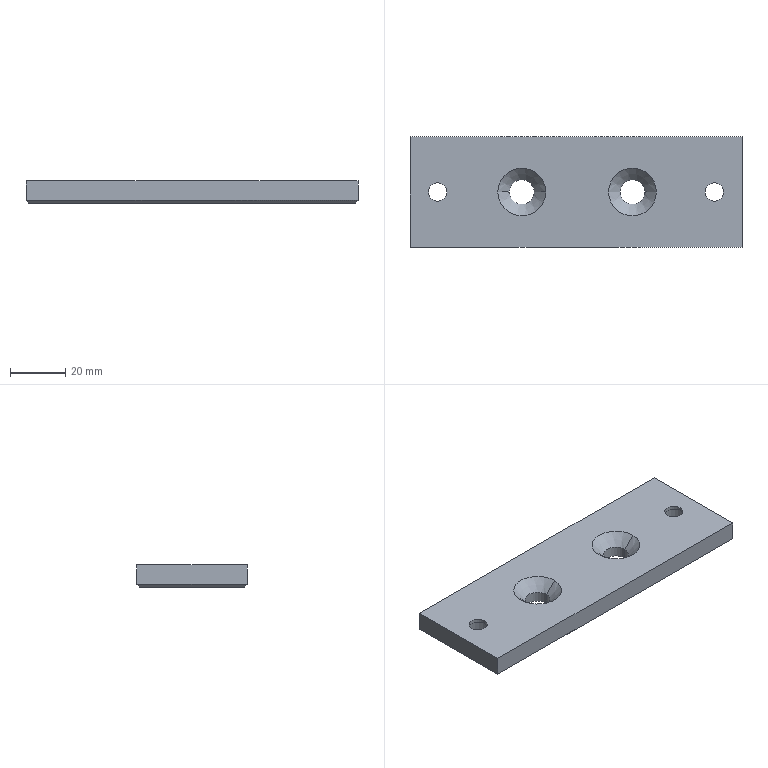Part | SolidWorks | features 3DProfileFeature 2, HoleWzd 2, Chamfer 1, Extrusion 1 | 1 solid | 28 faces | box 120 x 40 x 8 mm | volume 35212 mm3 | cylinder 12 | plane 12 | cone 4 | commonest cylinder face diameters 6.6 x4 9 x4 11 x4
STEP:
#1=CARTESIAN_POINT('',(55.5,0.,2.8));
#2=VERTEX_POINT('',#1);
#3=CARTESIAN_POINT('',(44.5,0.,2.8));
#4=VERTEX_POINT('',#3);
#5=CARTESIAN_POINT('',(50.,0.,2.8));
#6=DIRECTION('',(0.,0.,-1.));
#7=DIRECTION('',(-1.,0.,0.));
#8=AXIS2_PLACEMENT_3D('',#5,#6,#7);
#9=CIRCLE('',#8,5.5);
#10=EDGE_CURVE('',#2,#4,#9,.T.);
#11=ORIENTED_EDGE('',*,*,#10,.F.);
#12=CARTESIAN_POINT('',(55.5,0.,-4.));
#13=VERTEX_POINT('',#12);
#14=CARTESIAN_POINT('',(55.5,0.,-4.));
#15=DIRECTION('',(0.,0.,-1.));
#16=VECTOR('',#15,1000.);
#17=LINE('',#14,#16);
#18=EDGE_CURVE('',#2,#13,#17,.T.);
#19=ORIENTED_EDGE('',*,*,#18,.T.);
#20=CARTESIAN_POINT('',(44.5,0.,-4.));
#21=VERTEX_POINT('',#20);
#22=CARTESIAN_POINT('',(50.,0.,-4.));
#23=DIRECTION('',(0.,0.,-1.));
#24=DIRECTION('',(-1.,0.,0.));
#25=AXIS2_PLACEMENT_3D('',#22,#23,#24);
#26=CIRCLE('',#25,5.5);
#27=EDGE_CURVE('',#13,#21,#26,.T.);
#28=ORIENTED_EDGE('',*,*,#27,.T.);
#29=CARTESIAN_POINT('',(44.5,0.,-4.));
#30=DIRECTION('',(0.,0.,-1.));
#31=VECTOR('',#30,1000.);
#32=LINE('',#29,#31);
#33=EDGE_CURVE('',#4,#21,#32,.T.);
#34=ORIENTED_EDGE('',*,*,#33,.F.);
#35=EDGE_LOOP('',(#11,#19,#28,#34));
#36=FACE_OUTER_BOUND('',#35,.T.);
#37=CARTESIAN_POINT('',(50.,0.,-4.));
#38=DIRECTION('',(0.,0.,-1.));
#39=DIRECTION('',(-1.,0.,0.));
#40=AXIS2_PLACEMENT_3D('',#37,#38,#39);
#41=CYLINDRICAL_SURFACE('',#40,5.5);
#42=ADVANCED_FACE('',(#36),#41,.F.);
#43=CARTESIAN_POINT('',(46.7,0.,4.));
#44=VERTEX_POINT('',#43);
#45=CARTESIAN_POINT('',(53.3,0.,4.));
#46=VERTEX_POINT('',#45);
#47=CARTESIAN_POINT('',(50.,0.,4.));
#48=DIRECTION('',(0.,0.,1.));
#49=DIRECTION('',(1.,0.,0.));
#50=AXIS2_PLACEMENT_3D('',#47,#48,#49);
#51=CIRCLE('',#50,3.3);
#52=EDGE_CURVE('',#44,#46,#51,.T.);
#53=ORIENTED_EDGE('',*,*,#52,.T.);
#54=CARTESIAN_POINT('',(53.3,0.,2.8));
#55=VERTEX_POINT('',#54);
#56=CARTESIAN_POINT('',(53.3,0.,-4.));
#57=DIRECTION('',(0.,0.,-1.));
#58=VECTOR('',#57,1000.);
#59=LINE('',#56,#58);
#60=EDGE_CURVE('',#46,#55,#59,.T.);
#61=ORIENTED_EDGE('',*,*,#60,.T.);
#62=CARTESIAN_POINT('',(46.7,0.,2.8));
#63=VERTEX_POINT('',#62);
#64=CARTESIAN_POINT('',(50.,0.,2.8));
#65=DIRECTION('',(0.,0.,-1.));
#66=DIRECTION('',(-1.,0.,0.));
#67=AXIS2_PLACEMENT_3D('',#64,#65,#66);
#68=CIRCLE('',#67,3.3);
#69=EDGE_CURVE('',#55,#63,#68,.T.);
#70=ORIENTED_EDGE('',*,*,#69,.T.);
#71=CARTESIAN_POINT('',(46.7,0.,-4.));
#72=DIRECTION('',(0.,0.,-1.));
#73=VECTOR('',#72,1000.);
#74=LINE('',#71,#73);
#75=EDGE_CURVE('',#44,#63,#74,.T.);
#76=ORIENTED_EDGE('',*,*,#75,.F.);
#77=EDGE_LOOP('',(#53,#61,#70,#76));
#78=FACE_OUTER_BOUND('',#77,.T.);
#79=CARTESIAN_POINT('',(50.,0.,-4.));
#80=DIRECTION('',(0.,0.,-1.));
#81=DIRECTION('',(-1.,0.,0.));
#82=AXIS2_PLACEMENT_3D('',#79,#80,#81);
#83=CYLINDRICAL_SURFACE('',#82,3.3);
#84=ADVANCED_FACE('',(#78),#83,.F.);
#85=CARTESIAN_POINT('',(-44.5,0.,2.8));
#86=VERTEX_POINT('',#85);
#87=CARTESIAN_POINT('',(-55.5,0.,2.8));
#88=VERTEX_POINT('',#87);
#89=CARTESIAN_POINT('',(-50.,0.,2.8));
#90=DIRECTION('',(0.,0.,-1.));
#91=DIRECTION('',(-1.,0.,0.));
#92=AXIS2_PLACEMENT_3D('',#89,#90,#91);
#93=CIRCLE('',#92,5.5);
#94=EDGE_CURVE('',#86,#88,#93,.T.);
#95=ORIENTED_EDGE('',*,*,#94,.F.);
#96=CARTESIAN_POINT('',(-44.5,0.,-4.));
#97=VERTEX_POINT('',#96);
#98=CARTESIAN_POINT('',(-44.5,0.,-4.));
#99=DIRECTION('',(0.,0.,-1.));
#100=VECTOR('',#99,1000.);
#101=LINE('',#98,#100);
#102=EDGE_CURVE('',#86,#97,#101,.T.);
#103=ORIENTED_EDGE('',*,*,#102,.T.);
#104=CARTESIAN_POINT('',(-55.5,0.,-4.));
#105=VERTEX_POINT('',#104);
#106=CARTESIAN_POINT('',(-50.,0.,-4.));
#107=DIRECTION('',(0.,0.,-1.));
#108=DIRECTION('',(-1.,0.,0.));
#109=AXIS2_PLACEMENT_3D('',#106,#107,#108);
#110=CIRCLE('',#109,5.5);
#111=EDGE_CURVE('',#97,#105,#110,.T.);
#112=ORIENTED_EDGE('',*,*,#111,.T.);
#113=CARTESIAN_POINT('',(-55.5,0.,-4.));
#114=DIRECTION('',(0.,0.,-1.));
#115=VECTOR('',#114,1000.);
#116=LINE('',#113,#115);
#117=EDGE_CURVE('',#88,#105,#116,.T.);
#118=ORIENTED_EDGE('',*,*,#117,.F.);
#119=EDGE_LOOP('',(#95,#103,#112,#118));
#120=FACE_OUTER_BOUND('',#119,.T.);
#121=CARTESIAN_POINT('',(-50.,0.,-4.));
#122=DIRECTION('',(0.,0.,-1.));
#123=DIRECTION('',(-1.,0.,0.));
#124=AXIS2_PLACEMENT_3D('',#121,#122,#123);
#125=CYLINDRICAL_SURFACE('',#124,5.5);
#126=ADVANCED_FACE('',(#120),#125,.F.);
#127=CARTESIAN_POINT('',(-53.3,0.,4.));
#128=VERTEX_POINT('',#127);
#129=CARTESIAN_POINT('',(-46.7,0.,4.));
#130=VERTEX_POINT('',#129);
#131=CARTESIAN_POINT('',(-50.,0.,4.));
#132=DIRECTION('',(0.,0.,1.));
#133=DIRECTION('',(1.,0.,0.));
#134=AXIS2_PLACEMENT_3D('',#131,#132,#133);
#135=CIRCLE('',#134,3.3);
#136=EDGE_CURVE('',#128,#130,#135,.T.);
#137=ORIENTED_EDGE('',*,*,#136,.T.);
#138=CARTESIAN_POINT('',(-46.7,0.,2.8));
#139=VERTEX_POINT('',#138);
#140=CARTESIAN_POINT('',(-46.7,0.,-4.));
#141=DIRECTION('',(0.,0.,-1.));
#142=VECTOR('',#141,1000.);
#143=LINE('',#140,#142);
#144=EDGE_CURVE('',#130,#139,#143,.T.);
#145=ORIENTED_EDGE('',*,*,#144,.T.);
#146=CARTESIAN_POINT('',(-53.3,0.,2.8));
#147=VERTEX_POINT('',#146);
#148=CARTESIAN_POINT('',(-50.,0.,2.8));
#149=DIRECTION('',(0.,0.,-1.));
#150=DIRECTION('',(-1.,0.,0.));
#151=AXIS2_PLACEMENT_3D('',#148,#149,#150);
#152=CIRCLE('',#151,3.3);
#153=EDGE_CURVE('',#139,#147,#152,.T.);
#154=ORIENTED_EDGE('',*,*,#153,.T.);
#155=CARTESIAN_POINT('',(-53.3,0.,-4.));
#156=DIRECTION('',(0.,0.,-1.));
#157=VECTOR('',#156,1000.);
#158=LINE('',#155,#157);
#159=EDGE_CURVE('',#128,#147,#158,.T.);
#160=ORIENTED_EDGE('',*,*,#159,.F.);
#161=EDGE_LOOP('',(#137,#145,#154,#160));
#162=FACE_OUTER_BOUND('',#161,.T.);
#163=CARTESIAN_POINT('',(-50.,0.,-4.));
#164=DIRECTION('',(0.,0.,-1.));
#165=DIRECTION('',(-1.,0.,0.));
#166=AXIS2_PLACEMENT_3D('',#163,#164,#165);
#167=CYLINDRICAL_SURFACE('',#166,3.3);
#168=ADVANCED_FACE('',(#162),#167,.F.);
#169=CARTESIAN_POINT('',(-24.096,0.,-0.15));
#170=VERTEX_POINT('',#169);
#171=CARTESIAN_POINT('',(-15.096,0.,-0.15));
#172=VERTEX_POINT('',#171);
#173=CARTESIAN_POINT('',(-19.596,0.,-0.15));
#174=DIRECTION('',(0.,0.,1.));
#175=DIRECTION('',(1.,0.,0.));
#176=AXIS2_PLACEMENT_3D('',#173,#174,#175);
#177=CIRCLE('',#176,4.5);
#178=EDGE_CURVE('',#170,#172,#177,.T.);
#179=ORIENTED_EDGE('',*,*,#178,.F.);
#180=CARTESIAN_POINT('',(-28.246,0.,4.));
#181=VERTEX_POINT('',#180);
#182=CARTESIAN_POINT('',(-28.246,0.,4.));
#183=DIRECTION('',(-0.7071,0.,0.7071));
#184=VECTOR('',#183,1000.);
#185=LINE('',#182,#184);
#186=EDGE_CURVE('',#170,#181,#185,.T.);
#187=ORIENTED_EDGE('',*,*,#186,.T.);
#188=CARTESIAN_POINT('',(-10.946,0.,4.));
#189=VERTEX_POINT('',#188);
#190=CARTESIAN_POINT('',(-19.596,0.,4.));
#191=DIRECTION('',(0.,0.,1.));
#192=DIRECTION('',(1.,0.,0.));
#193=AXIS2_PLACEMENT_3D('',#190,#191,#192);
#194=CIRCLE('',#193,8.65);
#195=EDGE_CURVE('',#181,#189,#194,.T.);
#196=ORIENTED_EDGE('',*,*,#195,.T.);
#197=CARTESIAN_POINT('',(-10.946,0.,4.));
#198=DIRECTION('',(0.7071,0.,0.7071));
#199=VECTOR('',#198,1000.);
#200=LINE('',#197,#199);
#201=EDGE_CURVE('',#172,#189,#200,.T.);
#202=ORIENTED_EDGE('',*,*,#201,.F.);
#203=EDGE_LOOP('',(#179,#187,#196,#202));
#204=FACE_OUTER_BOUND('',#203,.T.);
#205=CARTESIAN_POINT('',(-19.596,0.,4.));
#206=DIRECTION('',(0.,0.,1.));
#207=DIRECTION('',(1.,0.,0.));
#208=AXIS2_PLACEMENT_3D('',#205,#206,#207);
#209=CONICAL_SURFACE('',#208,8.65,0.7854);
#210=ADVANCED_FACE('',(#204),#209,.F.);
#211=CARTESIAN_POINT('',(-24.096,0.,-4.));
#212=VERTEX_POINT('',#211);
#213=CARTESIAN_POINT('',(-15.096,0.,-4.));
#214=VERTEX_POINT('',#213);
#215=CARTESIAN_POINT('',(-19.596,0.,-4.));
#216=DIRECTION('',(0.,0.,1.));
#217=DIRECTION('',(1.,0.,0.));
#218=AXIS2_PLACEMENT_3D('',#215,#216,#217);
#219=CIRCLE('',#218,4.5);
#220=EDGE_CURVE('',#212,#214,#219,.T.);
#221=ORIENTED_EDGE('',*,*,#220,.F.);
#222=CARTESIAN_POINT('',(-24.096,0.,4.));
#223=DIRECTION('',(0.,0.,1.));
#224=VECTOR('',#223,1000.);
#225=LINE('',#222,#224);
#226=EDGE_CURVE('',#212,#170,#225,.T.);
#227=ORIENTED_EDGE('',*,*,#226,.T.);
#228=ORIENTED_EDGE('',*,*,#178,.T.);
#229=CARTESIAN_POINT('',(-15.096,0.,4.));
#230=DIRECTION('',(0.,0.,1.));
#231=VECTOR('',#230,1000.);
#232=LINE('',#229,#231);
#233=EDGE_CURVE('',#214,#172,#232,.T.);
#234=ORIENTED_EDGE('',*,*,#233,.F.);
#235=EDGE_LOOP('',(#221,#227,#228,#234));
#236=FACE_OUTER_BOUND('',#235,.T.);
#237=CARTESIAN_POINT('',(-19.596,0.,4.));
#238=DIRECTION('',(0.,0.,1.));
#239=DIRECTION('',(1.,0.,0.));
#240=AXIS2_PLACEMENT_3D('',#237,#238,#239);
#241=CYLINDRICAL_SURFACE('',#240,4.5);
#242=ADVANCED_FACE('',(#236),#241,.F.);
#243=CARTESIAN_POINT('',(15.904,0.,-0.15));
#244=VERTEX_POINT('',#243);
#245=CARTESIAN_POINT('',(24.904,0.,-0.15));
#246=VERTEX_POINT('',#245);
#247=CARTESIAN_POINT('',(20.404,0.,-0.15));
#248=DIRECTION('',(0.,0.,1.));
#249=DIRECTION('',(1.,0.,0.));
#250=AXIS2_PLACEMENT_3D('',#247,#248,#249);
#251=CIRCLE('',#250,4.5);
#252=EDGE_CURVE('',#244,#246,#251,.T.);
#253=ORIENTED_EDGE('',*,*,#252,.F.);
#254=CARTESIAN_POINT('',(11.754,0.,4.));
#255=VERTEX_POINT('',#254);
#256=CARTESIAN_POINT('',(11.754,0.,4.));
#257=DIRECTION('',(-0.7071,0.,0.7071));
#258=VECTOR('',#257,1000.);
#259=LINE('',#256,#258);
#260=EDGE_CURVE('',#244,#255,#259,.T.);
#261=ORIENTED_EDGE('',*,*,#260,.T.);
#262=CARTESIAN_POINT('',(29.054,0.,4.));
#263=VERTEX_POINT('',#262);
#264=CARTESIAN_POINT('',(20.404,0.,4.));
#265=DIRECTION('',(0.,0.,1.));
#266=DIRECTION('',(1.,0.,0.));
#267=AXIS2_PLACEMENT_3D('',#264,#265,#266);
#268=CIRCLE('',#267,8.65);
#269=EDGE_CURVE('',#255,#263,#268,.T.);
#270=ORIENTED_EDGE('',*,*,#269,.T.);
#271=CARTESIAN_POINT('',(29.054,0.,4.));
#272=DIRECTION('',(0.7071,0.,0.7071));
#273=VECTOR('',#272,1000.);
#274=LINE('',#271,#273);
#275=EDGE_CURVE('',#246,#263,#274,.T.);
#276=ORIENTED_EDGE('',*,*,#275,.F.);
#277=EDGE_LOOP('',(#253,#261,#270,#276));
#278=FACE_OUTER_BOUND('',#277,.T.);
#279=CARTESIAN_POINT('',(20.404,0.,4.));
#280=DIRECTION('',(0.,0.,1.));
#281=DIRECTION('',(1.,0.,0.));
#282=AXIS2_PLACEMENT_3D('',#279,#280,#281);
#283=CONICAL_SURFACE('',#282,8.65,0.7854);
#284=ADVANCED_FACE('',(#278),#283,.F.);
#285=CARTESIAN_POINT('',(15.904,0.,-4.));
#286=VERTEX_POINT('',#285);
#287=CARTESIAN_POINT('',(24.904,0.,-4.));
#288=VERTEX_POINT('',#287);
#289=CARTESIAN_POINT('',(20.404,0.,-4.));
#290=DIRECTION('',(0.,0.,1.));
#291=DIRECTION('',(1.,0.,0.));
#292=AXIS2_PLACEMENT_3D('',#289,#290,#291);
#293=CIRCLE('',#292,4.5);
#294=EDGE_CURVE('',#286,#288,#293,.T.);
#295=ORIENTED_EDGE('',*,*,#294,.F.);
#296=CARTESIAN_POINT('',(15.904,0.,4.));
#297=DIRECTION('',(0.,0.,1.));
#298=VECTOR('',#297,1000.);
#299=LINE('',#296,#298);
#300=EDGE_CURVE('',#286,#244,#299,.T.);
#301=ORIENTED_EDGE('',*,*,#300,.T.);
#302=ORIENTED_EDGE('',*,*,#252,.T.);
#303=CARTESIAN_POINT('',(24.904,0.,4.));
#304=DIRECTION('',(0.,0.,1.));
#305=VECTOR('',#304,1000.);
#306=LINE('',#303,#305);
#307=EDGE_CURVE('',#288,#246,#306,.T.);
#308=ORIENTED_EDGE('',*,*,#307,.F.);
#309=EDGE_LOOP('',(#295,#301,#302,#308));
#310=FACE_OUTER_BOUND('',#309,.T.);
#311=CARTESIAN_POINT('',(20.404,0.,4.));
#312=DIRECTION('',(0.,0.,1.));
#313=DIRECTION('',(1.,0.,0.));
#314=AXIS2_PLACEMENT_3D('',#311,#312,#313);
#315=CYLINDRICAL_SURFACE('',#314,4.5);
#316=ADVANCED_FACE('',(#310),#315,.F.);
#317=CARTESIAN_POINT('',(60.,-20.,4.));
#318=VERTEX_POINT('',#317);
#319=CARTESIAN_POINT('',(60.,-20.,-3.));
#320=VERTEX_POINT('',#319);
#321=CARTESIAN_POINT('',(60.,-20.,4.));
#322=DIRECTION('',(0.,0.,-1.));
#323=VECTOR('',#322,1000.);
#324=LINE('',#321,#323);
#325=EDGE_CURVE('',#318,#320,#324,.T.);
#326=ORIENTED_EDGE('',*,*,#325,.T.);
#327=CARTESIAN_POINT('',(60.,20.,-3.));
#328=VERTEX_POINT('',#327);
#329=CARTESIAN_POINT('',(60.,20.,-3.));
#330=DIRECTION('',(0.,1.,0.));
#331=VECTOR('',#330,1000.);
#332=LINE('',#329,#331);
#333=EDGE_CURVE('',#320,#328,#332,.T.);
#334=ORIENTED_EDGE('',*,*,#333,.T.);
#335=CARTESIAN_POINT('',(60.,20.,4.));
#336=VERTEX_POINT('',#335);
#337=CARTESIAN_POINT('',(60.,20.,4.));
#338=DIRECTION('',(0.,0.,-1.));
#339=VECTOR('',#338,1000.);
#340=LINE('',#337,#339);
#341=EDGE_CURVE('',#336,#328,#340,.T.);
#342=ORIENTED_EDGE('',*,*,#341,.F.);
#343=CARTESIAN_POINT('',(60.,20.,4.));
#344=DIRECTION('',(0.,1.,0.));
#345=VECTOR('',#344,1000.);
#346=LINE('',#343,#345);
#347=EDGE_CURVE('',#318,#336,#346,.T.);
#348=ORIENTED_EDGE('',*,*,#347,.F.);
#349=EDGE_LOOP('',(#326,#334,#342,#348));
#350=FACE_OUTER_BOUND('',#349,.T.);
#351=CARTESIAN_POINT('',(60.,20.,4.));
#352=DIRECTION('',(-1.,0.,0.));
#353=DIRECTION('',(0.,-1.,0.));
#354=AXIS2_PLACEMENT_3D('',#351,#352,#353);
#355=PLANE('',#354);
#356=ADVANCED_FACE('',(#350),#355,.F.);
#357=ORIENTED_EDGE('',*,*,#341,.T.);
#358=CARTESIAN_POINT('',(-60.,20.,-3.));
#359=VERTEX_POINT('',#358);
#360=CARTESIAN_POINT('',(-60.,20.,-3.));
#361=DIRECTION('',(-1.,0.,0.));
#362=VECTOR('',#361,1000.);
#363=LINE('',#360,#362);
#364=EDGE_CURVE('',#328,#359,#363,.T.);
#365=ORIENTED_EDGE('',*,*,#364,.T.);
#366=CARTESIAN_POINT('',(-60.,20.,4.));
#367=VERTEX_POINT('',#366);
#368=CARTESIAN_POINT('',(-60.,20.,4.));
#369=DIRECTION('',(0.,0.,-1.));
#370=VECTOR('',#369,1000.);
#371=LINE('',#368,#370);
#372=EDGE_CURVE('',#367,#359,#371,.T.);
#373=ORIENTED_EDGE('',*,*,#372,.F.);
#374=CARTESIAN_POINT('',(-60.,20.,4.));
#375=DIRECTION('',(-1.,0.,0.));
#376=VECTOR('',#375,1000.);
#377=LINE('',#374,#376);
#378=EDGE_CURVE('',#336,#367,#377,.T.);
#379=ORIENTED_EDGE('',*,*,#378,.F.);
#380=EDGE_LOOP('',(#357,#365,#373,#379));
#381=FACE_OUTER_BOUND('',#380,.T.);
#382=CARTESIAN_POINT('',(-60.,20.,4.));
#383=DIRECTION('',(0.,-1.,0.));
#384=DIRECTION('',(0.,0.,-1.));
#385=AXIS2_PLACEMENT_3D('',#382,#383,#384);
#386=PLANE('',#385);
#387=ADVANCED_FACE('',(#381),#386,.F.);
#388=ORIENTED_EDGE('',*,*,#372,.T.);
#389=CARTESIAN_POINT('',(-60.,-20.,-3.));
#390=VERTEX_POINT('',#389);
#391=CARTESIAN_POINT('',(-60.,20.,-3.));
#392=DIRECTION('',(0.,-1.,0.));
#393=VECTOR('',#392,1000.);
#394=LINE('',#391,#393);
#395=EDGE_CURVE('',#359,#390,#394,.T.);
#396=ORIENTED_EDGE('',*,*,#395,.T.);
#397=CARTESIAN_POINT('',(-60.,-20.,4.));
#398=VERTEX_POINT('',#397);
#399=CARTESIAN_POINT('',(-60.,-20.,4.));
#400=DIRECTION('',(0.,0.,-1.));
#401=VECTOR('',#400,1000.);
#402=LINE('',#399,#401);
#403=EDGE_CURVE('',#398,#390,#402,.T.);
#404=ORIENTED_EDGE('',*,*,#403,.F.);
#405=CARTESIAN_POINT('',(-60.,20.,4.));
#406=DIRECTION('',(0.,-1.,0.));
#407=VECTOR('',#406,1000.);
#408=LINE('',#405,#407);
#409=EDGE_CURVE('',#367,#398,#408,.T.);
#410=ORIENTED_EDGE('',*,*,#409,.F.);
#411=EDGE_LOOP('',(#388,#396,#404,#410));
#412=FACE_OUTER_BOUND('',#411,.T.);
#413=CARTESIAN_POINT('',(-60.,20.,4.));
#414=DIRECTION('',(1.,0.,0.));
#415=DIRECTION('',(0.,1.,0.));
#416=AXIS2_PLACEMENT_3D('',#413,#414,#415);
#417=PLANE('',#416);
#418=ADVANCED_FACE('',(#412),#417,.F.);
#419=ORIENTED_EDGE('',*,*,#403,.T.);
#420=CARTESIAN_POINT('',(-60.,-20.,-3.));
#421=DIRECTION('',(1.,0.,0.));
#422=VECTOR('',#421,1000.);
#423=LINE('',#420,#422);
#424=EDGE_CURVE('',#390,#320,#423,.T.);
#425=ORIENTED_EDGE('',*,*,#424,.T.);
#426=ORIENTED_EDGE('',*,*,#325,.F.);
#427=CARTESIAN_POINT('',(-60.,-20.,4.));
#428=DIRECTION('',(1.,0.,0.));
#429=VECTOR('',#428,1000.);
#430=LINE('',#427,#429);
#431=EDGE_CURVE('',#398,#318,#430,.T.);
#432=ORIENTED_EDGE('',*,*,#431,.F.);
#433=EDGE_LOOP('',(#419,#425,#426,#432));
#434=FACE_OUTER_BOUND('',#433,.T.);
#435=CARTESIAN_POINT('',(-60.,-20.,4.));
#436=DIRECTION('',(0.,1.,0.));
#437=DIRECTION('',(0.,0.,1.));
#438=AXIS2_PLACEMENT_3D('',#435,#436,#437);
#439=PLANE('',#438);
#440=ADVANCED_FACE('',(#434),#439,.F.);
#441=ORIENTED_EDGE('',*,*,#52,.F.);
#442=CARTESIAN_POINT('',(50.,0.,4.));
#443=DIRECTION('',(0.,0.,1.));
#444=DIRECTION('',(1.,0.,0.));
#445=AXIS2_PLACEMENT_3D('',#442,#443,#444);
#446=CIRCLE('',#445,3.3);
#447=EDGE_CURVE('',#46,#44,#446,.T.);
#448=ORIENTED_EDGE('',*,*,#447,.F.);
#449=EDGE_LOOP('',(#441,#448));
#450=FACE_BOUND('',#449,.T.);
#451=ORIENTED_EDGE('',*,*,#136,.F.);
#452=CARTESIAN_POINT('',(-50.,0.,4.));
#453=DIRECTION('',(0.,0.,1.));
#454=DIRECTION('',(1.,0.,0.));
#455=AXIS2_PLACEMENT_3D('',#452,#453,#454);
#456=CIRCLE('',#455,3.3);
#457=EDGE_CURVE('',#130,#128,#456,.T.);
#458=ORIENTED_EDGE('',*,*,#457,.F.);
#459=EDGE_LOOP('',(#451,#458));
#460=FACE_BOUND('',#459,.T.);
#461=CARTESIAN_POINT('',(-19.596,0.,4.));
#462=DIRECTION('',(0.,0.,1.));
#463=DIRECTION('',(1.,0.,0.));
#464=AXIS2_PLACEMENT_3D('',#461,#462,#463);
#465=CIRCLE('',#464,8.65);
#466=EDGE_CURVE('',#189,#181,#465,.T.);
#467=ORIENTED_EDGE('',*,*,#466,.F.);
#468=ORIENTED_EDGE('',*,*,#195,.F.);
#469=EDGE_LOOP('',(#467,#468));
#470=FACE_BOUND('',#469,.T.);
#471=CARTESIAN_POINT('',(20.404,0.,4.));
#472=DIRECTION('',(0.,0.,1.));
#473=DIRECTION('',(1.,0.,0.));
#474=AXIS2_PLACEMENT_3D('',#471,#472,#473);
#475=CIRCLE('',#474,8.65);
#476=EDGE_CURVE('',#263,#255,#475,.T.);
#477=ORIENTED_EDGE('',*,*,#476,.F.);
#478=ORIENTED_EDGE('',*,*,#269,.F.);
#479=EDGE_LOOP('',(#477,#478));
#480=FACE_BOUND('',#479,.T.);
#481=ORIENTED_EDGE('',*,*,#347,.T.);
#482=ORIENTED_EDGE('',*,*,#378,.T.);
#483=ORIENTED_EDGE('',*,*,#409,.T.);
#484=ORIENTED_EDGE('',*,*,#431,.T.);
#485=EDGE_LOOP('',(#481,#482,#483,#484));
#486=FACE_OUTER_BOUND('',#485,.T.);
#487=CARTESIAN_POINT('',(0.,0.,4.));
#488=DIRECTION('',(0.,0.,1.));
#489=DIRECTION('',(1.,0.,0.));
#490=AXIS2_PLACEMENT_3D('',#487,#488,#489);
#491=PLANE('',#490);
#492=ADVANCED_FACE('',(#450,#460,#470,#480,#486),#491,.T.);
#493=CARTESIAN_POINT('',(-59.,19.,-4.));
#494=VERTEX_POINT('',#493);
#495=CARTESIAN_POINT('',(59.,19.,-4.));
#496=VERTEX_POINT('',#495);
#497=CARTESIAN_POINT('',(0.,19.,-4.));
#498=DIRECTION('',(1.,0.,0.));
#499=VECTOR('',#498,1000.);
#500=LINE('',#497,#499);
#501=EDGE_CURVE('',#494,#496,#500,.T.);
#502=ORIENTED_EDGE('',*,*,#501,.T.);
#503=CARTESIAN_POINT('',(59.,-19.,-4.));
#504=VERTEX_POINT('',#503);
#505=CARTESIAN_POINT('',(59.,0.,-4.));
#506=DIRECTION('',(0.,-1.,0.));
#507=VECTOR('',#506,1000.);
#508=LINE('',#505,#507);
#509=EDGE_CURVE('',#496,#504,#508,.T.);
#510=ORIENTED_EDGE('',*,*,#509,.T.);
#511=CARTESIAN_POINT('',(-59.,-19.,-4.));
#512=VERTEX_POINT('',#511);
#513=CARTESIAN_POINT('',(0.,-19.,-4.));
#514=DIRECTION('',(-1.,0.,0.));
#515=VECTOR('',#514,1000.);
#516=LINE('',#513,#515);
#517=EDGE_CURVE('',#504,#512,#516,.T.);
#518=ORIENTED_EDGE('',*,*,#517,.T.);
#519=CARTESIAN_POINT('',(-59.,0.,-4.));
#520=DIRECTION('',(0.,1.,0.));
#521=VECTOR('',#520,1000.);
#522=LINE('',#519,#521);
#523=EDGE_CURVE('',#512,#494,#522,.T.);
#524=ORIENTED_EDGE('',*,*,#523,.T.);
#525=EDGE_LOOP('',(#502,#510,#518,#524));
#526=FACE_OUTER_BOUND('',#525,.T.);
#527=CARTESIAN_POINT('',(50.,0.,-4.));
#528=DIRECTION('',(0.,0.,-1.));
#529=DIRECTION('',(-1.,0.,0.));
#530=AXIS2_PLACEMENT_3D('',#527,#528,#529);
#531=CIRCLE('',#530,5.5);
#532=EDGE_CURVE('',#21,#13,#531,.T.);
#533=ORIENTED_EDGE('',*,*,#532,.F.);
#534=ORIENTED_EDGE('',*,*,#27,.F.);
#535=EDGE_LOOP('',(#533,#534));
#536=FACE_BOUND('',#535,.T.);
#537=CARTESIAN_POINT('',(-50.,0.,-4.));
#538=DIRECTION('',(0.,0.,-1.));
#539=DIRECTION('',(-1.,0.,0.));
#540=AXIS2_PLACEMENT_3D('',#537,#538,#539);
#541=CIRCLE('',#540,5.5);
#542=EDGE_CURVE('',#105,#97,#541,.T.);
#543=ORIENTED_EDGE('',*,*,#542,.F.);
#544=ORIENTED_EDGE('',*,*,#111,.F.);
#545=EDGE_LOOP('',(#543,#544));
#546=FACE_BOUND('',#545,.T.);
#547=CARTESIAN_POINT('',(-19.596,0.,-4.));
#548=DIRECTION('',(0.,0.,1.));
#549=DIRECTION('',(1.,0.,0.));
#550=AXIS2_PLACEMENT_3D('',#547,#548,#549);
#551=CIRCLE('',#550,4.5);
#552=EDGE_CURVE('',#214,#212,#551,.T.);
#553=ORIENTED_EDGE('',*,*,#552,.T.);
#554=ORIENTED_EDGE('',*,*,#220,.T.);
#555=EDGE_LOOP('',(#553,#554));
#556=FACE_BOUND('',#555,.T.);
#557=CARTESIAN_POINT('',(20.404,0.,-4.));
#558=DIRECTION('',(0.,0.,1.));
#559=DIRECTION('',(1.,0.,0.));
#560=AXIS2_PLACEMENT_3D('',#557,#558,#559);
#561=CIRCLE('',#560,4.5);
#562=EDGE_CURVE('',#288,#286,#561,.T.);
#563=ORIENTED_EDGE('',*,*,#562,.T.);
#564=ORIENTED_EDGE('',*,*,#294,.T.);
#565=EDGE_LOOP('',(#563,#564));
#566=FACE_BOUND('',#565,.T.);
#567=CARTESIAN_POINT('',(0.,0.,-4.));
#568=DIRECTION('',(0.,0.,1.));
#569=DIRECTION('',(1.,0.,0.));
#570=AXIS2_PLACEMENT_3D('',#567,#568,#569);
#571=PLANE('',#570);
#572=ADVANCED_FACE('',(#526,#536,#546,#556,#566),#571,.F.);
#573=ORIENTED_EDGE('',*,*,#300,.F.);
#574=ORIENTED_EDGE('',*,*,#562,.F.);
#575=ORIENTED_EDGE('',*,*,#307,.T.);
#576=CARTESIAN_POINT('',(20.404,0.,-0.15));
#577=DIRECTION('',(0.,0.,1.));
#578=DIRECTION('',(1.,0.,0.));
#579=AXIS2_PLACEMENT_3D('',#576,#577,#578);
#580=CIRCLE('',#579,4.5);
#581=EDGE_CURVE('',#246,#244,#580,.T.);
#582=ORIENTED_EDGE('',*,*,#581,.T.);
#583=EDGE_LOOP('',(#573,#574,#575,#582));
#584=FACE_OUTER_BOUND('',#583,.T.);
#585=CARTESIAN_POINT('',(20.404,0.,4.));
#586=DIRECTION('',(0.,0.,1.));
#587=DIRECTION('',(1.,0.,0.));
#588=AXIS2_PLACEMENT_3D('',#585,#586,#587);
#589=CYLINDRICAL_SURFACE('',#588,4.5);
#590=ADVANCED_FACE('',(#584),#589,.F.);
#591=ORIENTED_EDGE('',*,*,#260,.F.);
#592=ORIENTED_EDGE('',*,*,#581,.F.);
#593=ORIENTED_EDGE('',*,*,#275,.T.);
#594=ORIENTED_EDGE('',*,*,#476,.T.);
#595=EDGE_LOOP('',(#591,#592,#593,#594));
#596=FACE_OUTER_BOUND('',#595,.T.);
#597=CARTESIAN_POINT('',(20.404,0.,4.));
#598=DIRECTION('',(0.,0.,1.));
#599=DIRECTION('',(1.,0.,0.));
#600=AXIS2_PLACEMENT_3D('',#597,#598,#599);
#601=CONICAL_SURFACE('',#600,8.65,0.7854);
#602=ADVANCED_FACE('',(#596),#601,.F.);
#603=ORIENTED_EDGE('',*,*,#226,.F.);
#604=ORIENTED_EDGE('',*,*,#552,.F.);
#605=ORIENTED_EDGE('',*,*,#233,.T.);
#606=CARTESIAN_POINT('',(-19.596,0.,-0.15));
#607=DIRECTION('',(0.,0.,1.));
#608=DIRECTION('',(1.,0.,0.));
#609=AXIS2_PLACEMENT_3D('',#606,#607,#608);
#610=CIRCLE('',#609,4.5);
#611=EDGE_CURVE('',#172,#170,#610,.T.);
#612=ORIENTED_EDGE('',*,*,#611,.T.);
#613=EDGE_LOOP('',(#603,#604,#605,#612));
#614=FACE_OUTER_BOUND('',#613,.T.);
#615=CARTESIAN_POINT('',(-19.596,0.,4.));
#616=DIRECTION('',(0.,0.,1.));
#617=DIRECTION('',(1.,0.,0.));
#618=AXIS2_PLACEMENT_3D('',#615,#616,#617);
#619=CYLINDRICAL_SURFACE('',#618,4.5);
#620=ADVANCED_FACE('',(#614),#619,.F.);
#621=ORIENTED_EDGE('',*,*,#186,.F.);
#622=ORIENTED_EDGE('',*,*,#611,.F.);
#623=ORIENTED_EDGE('',*,*,#201,.T.);
#624=ORIENTED_EDGE('',*,*,#466,.T.);
#625=EDGE_LOOP('',(#621,#622,#623,#624));
#626=FACE_OUTER_BOUND('',#625,.T.);
#627=CARTESIAN_POINT('',(-19.596,0.,4.));
#628=DIRECTION('',(0.,0.,1.));
#629=DIRECTION('',(1.,0.,0.));
#630=AXIS2_PLACEMENT_3D('',#627,#628,#629);
#631=CONICAL_SURFACE('',#630,8.65,0.7854);
#632=ADVANCED_FACE('',(#626),#631,.F.);
#633=ORIENTED_EDGE('',*,*,#144,.F.);
#634=ORIENTED_EDGE('',*,*,#457,.T.);
#635=ORIENTED_EDGE('',*,*,#159,.T.);
#636=CARTESIAN_POINT('',(-50.,0.,2.8));
#637=DIRECTION('',(0.,0.,-1.));
#638=DIRECTION('',(-1.,0.,0.));
#639=AXIS2_PLACEMENT_3D('',#636,#637,#638);
#640=CIRCLE('',#639,3.3);
#641=EDGE_CURVE('',#147,#139,#640,.T.);
#642=ORIENTED_EDGE('',*,*,#641,.T.);
#643=EDGE_LOOP('',(#633,#634,#635,#642));
#644=FACE_OUTER_BOUND('',#643,.T.);
#645=CARTESIAN_POINT('',(-50.,0.,-4.));
#646=DIRECTION('',(0.,0.,-1.));
#647=DIRECTION('',(-1.,0.,0.));
#648=AXIS2_PLACEMENT_3D('',#645,#646,#647);
#649=CYLINDRICAL_SURFACE('',#648,3.3);
#650=ADVANCED_FACE('',(#644),#649,.F.);
#651=ORIENTED_EDGE('',*,*,#641,.F.);
#652=ORIENTED_EDGE('',*,*,#153,.F.);
#653=EDGE_LOOP('',(#651,#652));
#654=FACE_BOUND('',#653,.T.);
#655=CARTESIAN_POINT('',(-50.,0.,2.8));
#656=DIRECTION('',(0.,0.,-1.));
#657=DIRECTION('',(-1.,0.,0.));
#658=AXIS2_PLACEMENT_3D('',#655,#656,#657);
#659=CIRCLE('',#658,5.5);
#660=EDGE_CURVE('',#88,#86,#659,.T.);
#661=ORIENTED_EDGE('',*,*,#660,.T.);
#662=ORIENTED_EDGE('',*,*,#94,.T.);
#663=EDGE_LOOP('',(#661,#662));
#664=FACE_OUTER_BOUND('',#663,.T.);
#665=CARTESIAN_POINT('',(-46.7,0.,2.8));
#666=DIRECTION('',(0.,0.,1.));
#667=DIRECTION('',(1.,0.,0.));
#668=AXIS2_PLACEMENT_3D('',#665,#666,#667);
#669=PLANE('',#668);
#670=ADVANCED_FACE('',(#654,#664),#669,.F.);
#671=ORIENTED_EDGE('',*,*,#102,.F.);
#672=ORIENTED_EDGE('',*,*,#660,.F.);
#673=ORIENTED_EDGE('',*,*,#117,.T.);
#674=ORIENTED_EDGE('',*,*,#542,.T.);
#675=EDGE_LOOP('',(#671,#672,#673,#674));
#676=FACE_OUTER_BOUND('',#675,.T.);
#677=CARTESIAN_POINT('',(-50.,0.,-4.));
#678=DIRECTION('',(0.,0.,-1.));
#679=DIRECTION('',(-1.,0.,0.));
#680=AXIS2_PLACEMENT_3D('',#677,#678,#679);
#681=CYLINDRICAL_SURFACE('',#680,5.5);
#682=ADVANCED_FACE('',(#676),#681,.F.);
#683=ORIENTED_EDGE('',*,*,#60,.F.);
#684=ORIENTED_EDGE('',*,*,#447,.T.);
#685=ORIENTED_EDGE('',*,*,#75,.T.);
#686=CARTESIAN_POINT('',(50.,0.,2.8));
#687=DIRECTION('',(0.,0.,-1.));
#688=DIRECTION('',(-1.,0.,0.));
#689=AXIS2_PLACEMENT_3D('',#686,#687,#688);
#690=CIRCLE('',#689,3.3);
#691=EDGE_CURVE('',#63,#55,#690,.T.);
#692=ORIENTED_EDGE('',*,*,#691,.T.);
#693=EDGE_LOOP('',(#683,#684,#685,#692));
#694=FACE_OUTER_BOUND('',#693,.T.);
#695=CARTESIAN_POINT('',(50.,0.,-4.));
#696=DIRECTION('',(0.,0.,-1.));
#697=DIRECTION('',(-1.,0.,0.));
#698=AXIS2_PLACEMENT_3D('',#695,#696,#697);
#699=CYLINDRICAL_SURFACE('',#698,3.3);
#700=ADVANCED_FACE('',(#694),#699,.F.);
#701=ORIENTED_EDGE('',*,*,#691,.F.);
#702=ORIENTED_EDGE('',*,*,#69,.F.);
#703=EDGE_LOOP('',(#701,#702));
#704=FACE_BOUND('',#703,.T.);
#705=CARTESIAN_POINT('',(50.,0.,2.8));
#706=DIRECTION('',(0.,0.,-1.));
#707=DIRECTION('',(-1.,0.,0.));
#708=AXIS2_PLACEMENT_3D('',#705,#706,#707);
#709=CIRCLE('',#708,5.5);
#710=EDGE_CURVE('',#4,#2,#709,.T.);
#711=ORIENTED_EDGE('',*,*,#710,.T.);
#712=ORIENTED_EDGE('',*,*,#10,.T.);
#713=EDGE_LOOP('',(#711,#712));
#714=FACE_OUTER_BOUND('',#713,.T.);
#715=CARTESIAN_POINT('',(53.3,0.,2.8));
#716=DIRECTION('',(0.,0.,1.));
#717=DIRECTION('',(1.,0.,0.));
#718=AXIS2_PLACEMENT_3D('',#715,#716,#717);
#719=PLANE('',#718);
#720=ADVANCED_FACE('',(#704,#714),#719,.F.);
#721=ORIENTED_EDGE('',*,*,#18,.F.);
#722=ORIENTED_EDGE('',*,*,#710,.F.);
#723=ORIENTED_EDGE('',*,*,#33,.T.);
#724=ORIENTED_EDGE('',*,*,#532,.T.);
#725=EDGE_LOOP('',(#721,#722,#723,#724));
#726=FACE_OUTER_BOUND('',#725,.T.);
#727=CARTESIAN_POINT('',(50.,0.,-4.));
#728=DIRECTION('',(0.,0.,-1.));
#729=DIRECTION('',(-1.,0.,0.));
#730=AXIS2_PLACEMENT_3D('',#727,#728,#729);
#731=CYLINDRICAL_SURFACE('',#730,5.5);
#732=ADVANCED_FACE('',(#726),#731,.F.);
#733=CARTESIAN_POINT('',(-60.,20.,-3.));
#734=DIRECTION('',(-0.5774,0.5774,0.5774));
#735=VECTOR('',#734,1000.);
#736=LINE('',#733,#735);
#737=EDGE_CURVE('',#494,#359,#736,.T.);
#738=ORIENTED_EDGE('',*,*,#737,.F.);
#739=ORIENTED_EDGE('',*,*,#523,.F.);
#740=CARTESIAN_POINT('',(-46.667,-6.667,-16.333));
#741=DIRECTION('',(0.5774,0.5774,-0.5774));
#742=VECTOR('',#741,1000.);
#743=LINE('',#740,#742);
#744=EDGE_CURVE('',#390,#512,#743,.T.);
#745=ORIENTED_EDGE('',*,*,#744,.F.);
#746=ORIENTED_EDGE('',*,*,#395,.F.);
#747=EDGE_LOOP('',(#738,#739,#745,#746));
#748=FACE_OUTER_BOUND('',#747,.T.);
#749=CARTESIAN_POINT('',(-60.,20.,-3.));
#750=DIRECTION('',(0.7071,0.,0.7071));
#751=DIRECTION('',(0.,-1.,0.));
#752=AXIS2_PLACEMENT_3D('',#749,#750,#751);
#753=PLANE('',#752);
#754=ADVANCED_FACE('',(#748),#753,.F.);
#755=ORIENTED_EDGE('',*,*,#744,.T.);
#756=ORIENTED_EDGE('',*,*,#517,.F.);
#757=CARTESIAN_POINT('',(20.,20.,-43.));
#758=DIRECTION('',(-0.5774,0.5774,-0.5774));
#759=VECTOR('',#758,1000.);
#760=LINE('',#757,#759);
#761=EDGE_CURVE('',#320,#504,#760,.T.);
#762=ORIENTED_EDGE('',*,*,#761,.F.);
#763=ORIENTED_EDGE('',*,*,#424,.F.);
#764=EDGE_LOOP('',(#755,#756,#762,#763));
#765=FACE_OUTER_BOUND('',#764,.T.);
#766=CARTESIAN_POINT('',(-60.,-20.,-3.));
#767=DIRECTION('',(0.,0.7071,0.7071));
#768=DIRECTION('',(1.,0.,0.));
#769=AXIS2_PLACEMENT_3D('',#766,#767,#768);
#770=PLANE('',#769);
#771=ADVANCED_FACE('',(#765),#770,.F.);
#772=ORIENTED_EDGE('',*,*,#737,.T.);
#773=ORIENTED_EDGE('',*,*,#364,.F.);
#774=CARTESIAN_POINT('',(20.,-20.,-43.));
#775=DIRECTION('',(0.5774,0.5774,0.5774));
#776=VECTOR('',#775,1000.);
#777=LINE('',#774,#776);
#778=EDGE_CURVE('',#496,#328,#777,.T.);
#779=ORIENTED_EDGE('',*,*,#778,.F.);
#780=ORIENTED_EDGE('',*,*,#501,.F.);
#781=EDGE_LOOP('',(#772,#773,#779,#780));
#782=FACE_OUTER_BOUND('',#781,.T.);
#783=CARTESIAN_POINT('',(-60.,20.,-3.));
#784=DIRECTION('',(0.,-0.7071,0.7071));
#785=DIRECTION('',(-1.,0.,0.));
#786=AXIS2_PLACEMENT_3D('',#783,#784,#785);
#787=PLANE('',#786);
#788=ADVANCED_FACE('',(#782),#787,.F.);
#789=ORIENTED_EDGE('',*,*,#761,.T.);
#790=ORIENTED_EDGE('',*,*,#509,.F.);
#791=ORIENTED_EDGE('',*,*,#778,.T.);
#792=ORIENTED_EDGE('',*,*,#333,.F.);
#793=EDGE_LOOP('',(#789,#790,#791,#792));
#794=FACE_OUTER_BOUND('',#793,.T.);
#795=CARTESIAN_POINT('',(60.,20.,-3.));
#796=DIRECTION('',(-0.7071,0.,0.7071));
#797=DIRECTION('',(0.,1.,0.));
#798=AXIS2_PLACEMENT_3D('',#795,#796,#797);
#799=PLANE('',#798);
#800=ADVANCED_FACE('',(#794),#799,.F.);
#801=CLOSED_SHELL('',(#42,#84,#126,#168,#210,#242,#284,#316,#356,#387,#418,#440,#492,#572,#590,#602,#620,#632,#650,#670,#682,#700,#720,#732,#754,#771,#788,#800));
#802=MANIFOLD_SOLID_BREP('',#801);
#803=CARTESIAN_POINT('',(0.,0.,0.));
#804=DIRECTION('',(0.,0.,1.));
#805=DIRECTION('',(1.,0.,0.));
#806=AXIS2_PLACEMENT_3D('',#803,#804,#805);
#807=(LENGTH_UNIT()NAMED_UNIT(*)SI_UNIT(.MILLI.,.METRE.));
#808=UNCERTAINTY_MEASURE_WITH_UNIT(LENGTH_MEASURE(0.00001),#807,'','');
#809=(NAMED_UNIT(*)PLANE_ANGLE_UNIT()SI_UNIT($,.RADIAN.));
#810=(NAMED_UNIT(*)SI_UNIT($,.STERADIAN.)SOLID_ANGLE_UNIT());
#811=(GEOMETRIC_REPRESENTATION_CONTEXT(3)GLOBAL_UNCERTAINTY_ASSIGNED_CONTEXT((#808))GLOBAL_UNIT_ASSIGNED_CONTEXT((#807,#809,#810))REPRESENTATION_CONTEXT('',''));
#812=ADVANCED_BREP_SHAPE_REPRESENTATION('',(#802,#806),#811);